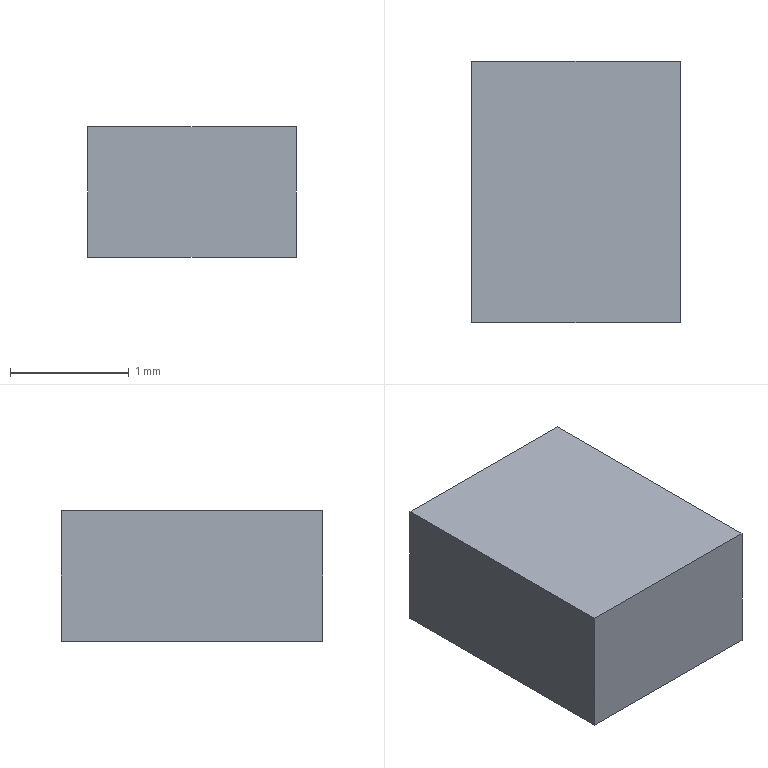Part | Creo | 1 solid | 6 faces | box 1.75 x 2.2 x 1.1 mm | volume 4.235 mm3 | plane 6
STEP:
#1=CARTESIAN_POINT('',(0.,0.,0.));
#2=DIRECTION('',(0.,0.,1.));
#3=DIRECTION('',(1.,0.,0.));
#4=AXIS2_PLACEMENT_3D('',#1,#2,#3);
#5=CARTESIAN_POINT('',(-0.875,-1.1,0.));
#6=VERTEX_POINT('',#5);
#7=CARTESIAN_POINT('',(0.875,-1.1,0.));
#8=VERTEX_POINT('',#7);
#9=CARTESIAN_POINT('',(-0.875,-1.1,0.));
#10=DIRECTION('',(1.,0.,0.));
#11=VECTOR('',#10,1.75);
#12=LINE('',#9,#11);
#13=EDGE_CURVE('',#6,#8,#12,.T.);
#14=ORIENTED_EDGE('',*,*,#13,.T.);
#15=CARTESIAN_POINT('',(0.875,1.1,0.));
#16=VERTEX_POINT('',#15);
#17=CARTESIAN_POINT('',(0.875,-1.1,0.));
#18=DIRECTION('',(0.,1.,0.));
#19=VECTOR('',#18,2.2);
#20=LINE('',#17,#19);
#21=EDGE_CURVE('',#8,#16,#20,.T.);
#22=ORIENTED_EDGE('',*,*,#21,.T.);
#23=CARTESIAN_POINT('',(-0.875,1.1,0.));
#24=VERTEX_POINT('',#23);
#25=CARTESIAN_POINT('',(0.875,1.1,0.));
#26=DIRECTION('',(-1.,0.,0.));
#27=VECTOR('',#26,1.75);
#28=LINE('',#25,#27);
#29=EDGE_CURVE('',#16,#24,#28,.T.);
#30=ORIENTED_EDGE('',*,*,#29,.T.);
#31=CARTESIAN_POINT('',(-0.875,1.1,0.));
#32=DIRECTION('',(0.,-1.,0.));
#33=VECTOR('',#32,2.2);
#34=LINE('',#31,#33);
#35=EDGE_CURVE('',#24,#6,#34,.T.);
#36=ORIENTED_EDGE('',*,*,#35,.T.);
#37=EDGE_LOOP('',(#14,#22,#30,#36));
#38=FACE_OUTER_BOUND('',#37,.F.);
#39=CARTESIAN_POINT('',(0.,0.,0.));
#40=DIRECTION('',(0.,0.,1.));
#41=DIRECTION('',(1.,0.,0.));
#42=AXIS2_PLACEMENT_3D('',#39,#40,#41);
#43=PLANE('',#42);
#44=ADVANCED_FACE('',(#38),#43,.F.);
#45=ORIENTED_EDGE('',*,*,#13,.F.);
#46=CARTESIAN_POINT('',(-0.875,-1.1,1.1));
#47=VERTEX_POINT('',#46);
#48=CARTESIAN_POINT('',(-0.875,-1.1,0.));
#49=DIRECTION('',(0.,0.,1.));
#50=VECTOR('',#49,1.1);
#51=LINE('',#48,#50);
#52=EDGE_CURVE('',#6,#47,#51,.T.);
#53=ORIENTED_EDGE('',*,*,#52,.T.);
#54=CARTESIAN_POINT('',(0.875,-1.1,1.1));
#55=VERTEX_POINT('',#54);
#56=CARTESIAN_POINT('',(-0.875,-1.1,1.1));
#57=DIRECTION('',(1.,0.,0.));
#58=VECTOR('',#57,1.75);
#59=LINE('',#56,#58);
#60=EDGE_CURVE('',#47,#55,#59,.T.);
#61=ORIENTED_EDGE('',*,*,#60,.T.);
#62=CARTESIAN_POINT('',(0.875,-1.1,0.));
#63=DIRECTION('',(0.,0.,1.));
#64=VECTOR('',#63,1.1);
#65=LINE('',#62,#64);
#66=EDGE_CURVE('',#8,#55,#65,.T.);
#67=ORIENTED_EDGE('',*,*,#66,.F.);
#68=EDGE_LOOP('',(#45,#53,#61,#67));
#69=FACE_OUTER_BOUND('',#68,.F.);
#70=CARTESIAN_POINT('',(-0.875,-1.1,0.));
#71=DIRECTION('',(0.,-1.,0.));
#72=DIRECTION('',(1.,0.,0.));
#73=AXIS2_PLACEMENT_3D('',#70,#71,#72);
#74=PLANE('',#73);
#75=ADVANCED_FACE('',(#69),#74,.T.);
#76=ORIENTED_EDGE('',*,*,#35,.F.);
#77=CARTESIAN_POINT('',(-0.875,1.1,1.1));
#78=VERTEX_POINT('',#77);
#79=CARTESIAN_POINT('',(-0.875,1.1,0.));
#80=DIRECTION('',(0.,0.,1.));
#81=VECTOR('',#80,1.1);
#82=LINE('',#79,#81);
#83=EDGE_CURVE('',#24,#78,#82,.T.);
#84=ORIENTED_EDGE('',*,*,#83,.T.);
#85=CARTESIAN_POINT('',(-0.875,1.1,1.1));
#86=DIRECTION('',(0.,-1.,0.));
#87=VECTOR('',#86,2.2);
#88=LINE('',#85,#87);
#89=EDGE_CURVE('',#78,#47,#88,.T.);
#90=ORIENTED_EDGE('',*,*,#89,.T.);
#91=ORIENTED_EDGE('',*,*,#52,.F.);
#92=EDGE_LOOP('',(#76,#84,#90,#91));
#93=FACE_OUTER_BOUND('',#92,.F.);
#94=CARTESIAN_POINT('',(-0.875,1.1,0.));
#95=DIRECTION('',(-1.,0.,0.));
#96=DIRECTION('',(0.,-1.,0.));
#97=AXIS2_PLACEMENT_3D('',#94,#95,#96);
#98=PLANE('',#97);
#99=ADVANCED_FACE('',(#93),#98,.T.);
#100=ORIENTED_EDGE('',*,*,#29,.F.);
#101=CARTESIAN_POINT('',(0.875,1.1,1.1));
#102=VERTEX_POINT('',#101);
#103=CARTESIAN_POINT('',(0.875,1.1,0.));
#104=DIRECTION('',(0.,0.,1.));
#105=VECTOR('',#104,1.1);
#106=LINE('',#103,#105);
#107=EDGE_CURVE('',#16,#102,#106,.T.);
#108=ORIENTED_EDGE('',*,*,#107,.T.);
#109=CARTESIAN_POINT('',(0.875,1.1,1.1));
#110=DIRECTION('',(-1.,0.,0.));
#111=VECTOR('',#110,1.75);
#112=LINE('',#109,#111);
#113=EDGE_CURVE('',#102,#78,#112,.T.);
#114=ORIENTED_EDGE('',*,*,#113,.T.);
#115=ORIENTED_EDGE('',*,*,#83,.F.);
#116=EDGE_LOOP('',(#100,#108,#114,#115));
#117=FACE_OUTER_BOUND('',#116,.F.);
#118=CARTESIAN_POINT('',(0.875,1.1,0.));
#119=DIRECTION('',(0.,1.,0.));
#120=DIRECTION('',(-1.,0.,0.));
#121=AXIS2_PLACEMENT_3D('',#118,#119,#120);
#122=PLANE('',#121);
#123=ADVANCED_FACE('',(#117),#122,.T.);
#124=ORIENTED_EDGE('',*,*,#21,.F.);
#125=ORIENTED_EDGE('',*,*,#66,.T.);
#126=CARTESIAN_POINT('',(0.875,-1.1,1.1));
#127=DIRECTION('',(0.,1.,0.));
#128=VECTOR('',#127,2.2);
#129=LINE('',#126,#128);
#130=EDGE_CURVE('',#55,#102,#129,.T.);
#131=ORIENTED_EDGE('',*,*,#130,.T.);
#132=ORIENTED_EDGE('',*,*,#107,.F.);
#133=EDGE_LOOP('',(#124,#125,#131,#132));
#134=FACE_OUTER_BOUND('',#133,.F.);
#135=CARTESIAN_POINT('',(0.875,-1.1,0.));
#136=DIRECTION('',(1.,0.,0.));
#137=DIRECTION('',(0.,1.,0.));
#138=AXIS2_PLACEMENT_3D('',#135,#136,#137);
#139=PLANE('',#138);
#140=ADVANCED_FACE('',(#134),#139,.T.);
#141=ORIENTED_EDGE('',*,*,#60,.F.);
#142=ORIENTED_EDGE('',*,*,#89,.F.);
#143=ORIENTED_EDGE('',*,*,#113,.F.);
#144=ORIENTED_EDGE('',*,*,#130,.F.);
#145=EDGE_LOOP('',(#141,#142,#143,#144));
#146=FACE_OUTER_BOUND('',#145,.F.);
#147=CARTESIAN_POINT('',(0.,0.,1.1));
#148=DIRECTION('',(0.,0.,1.));
#149=DIRECTION('',(1.,0.,0.));
#150=AXIS2_PLACEMENT_3D('',#147,#148,#149);
#151=PLANE('',#150);
#152=ADVANCED_FACE('',(#146),#151,.T.);
#153=CLOSED_SHELL('',(#44,#75,#99,#123,#140,#152));
#154=MANIFOLD_SOLID_BREP('',#153);
#155=(LENGTH_UNIT()NAMED_UNIT(*)SI_UNIT(.MILLI.,.METRE.));
#156=UNCERTAINTY_MEASURE_WITH_UNIT(LENGTH_MEASURE(0.0003019),#155,'','');
#157=(NAMED_UNIT(*)PLANE_ANGLE_UNIT()SI_UNIT($,.RADIAN.));
#158=PLANE_ANGLE_MEASURE_WITH_UNIT(PLANE_ANGLE_MEASURE(0.01745),#157);
#159=(CONVERSION_BASED_UNIT('DEGREE',#158)NAMED_UNIT(*)PLANE_ANGLE_UNIT());
#160=(NAMED_UNIT(*)SI_UNIT($,.STERADIAN.)SOLID_ANGLE_UNIT());
#161=(GEOMETRIC_REPRESENTATION_CONTEXT(3)GLOBAL_UNCERTAINTY_ASSIGNED_CONTEXT((#156))GLOBAL_UNIT_ASSIGNED_CONTEXT((#155,#159,#160))REPRESENTATION_CONTEXT('',''));
#162=ADVANCED_BREP_SHAPE_REPRESENTATION('',(#4,#154),#161);